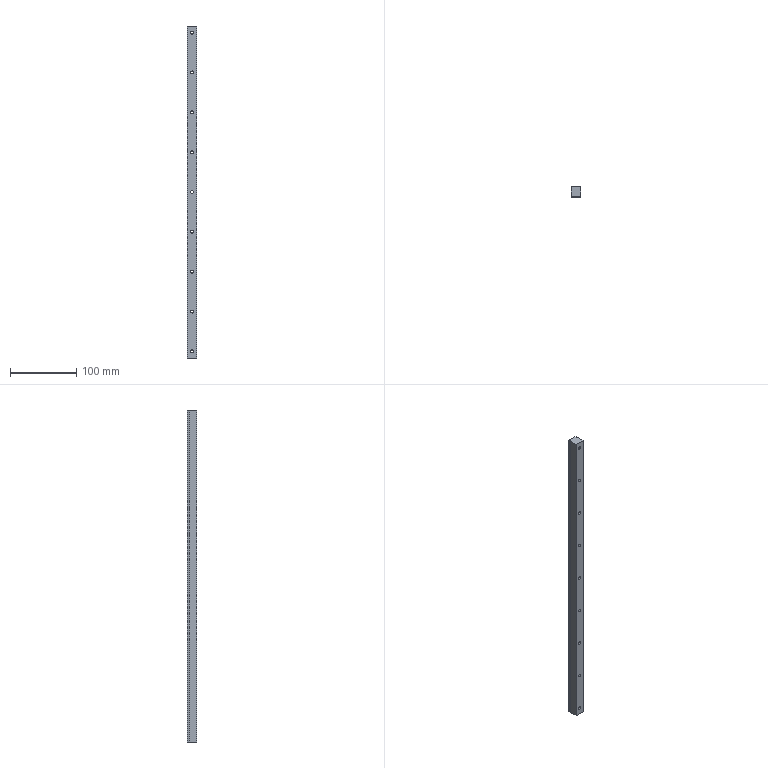Part | STEP file | 1 solid | 37 faces | box 15 x 15 x 500 mm | volume 107236 mm3 | cylinder 20 | plane 17 | commonest cylinder face diameters 4.5 x9 8 x9 2 x2